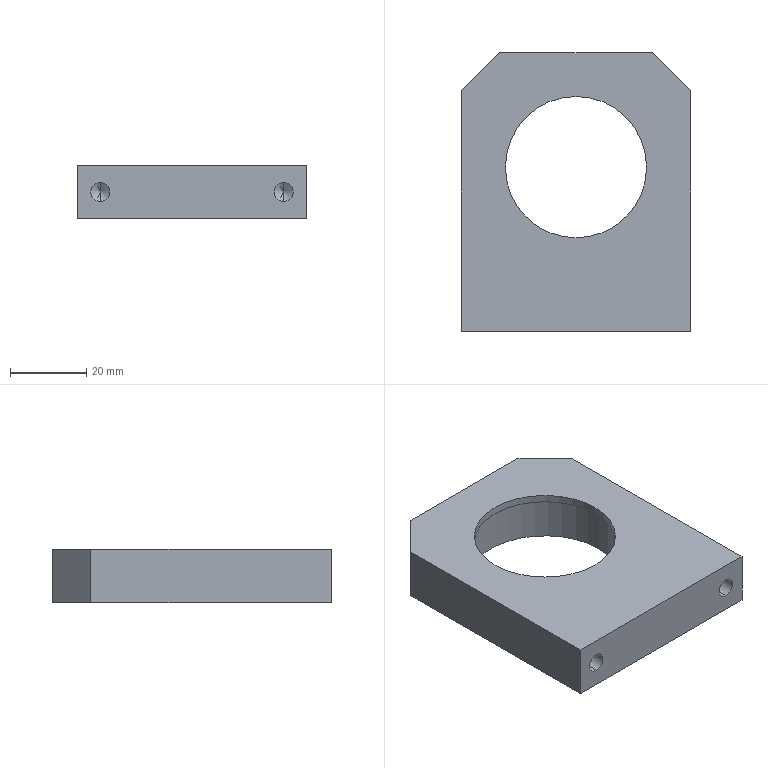Part | SolidWorks | features 3DProfileFeature 1, Chamfer 1, Extrusion 1, HoleWzd 1, ICE 1 | 1 solid | 21 faces | box 60 x 73 x 14 mm | volume 42120 mm3 | plane 9 | cylinder 8 | cone 4 | commonest cylinder face diameters 5 x4 37 x2 40 x2
STEP:
#1=CARTESIAN_POINT('',(-24.,-22.5,2.5));
#2=VERTEX_POINT('',#1);
#3=CARTESIAN_POINT('',(-24.,-22.5,-2.5));
#4=VERTEX_POINT('',#3);
#5=CARTESIAN_POINT('',(-24.,-22.5,0.));
#6=DIRECTION('',(0.,-1.,0.));
#7=DIRECTION('',(0.,0.,-1.));
#8=AXIS2_PLACEMENT_3D('',#5,#6,#7);
#9=CIRCLE('',#8,2.5);
#10=EDGE_CURVE('',#2,#4,#9,.T.);
#11=ORIENTED_EDGE('',*,*,#10,.F.);
#12=CARTESIAN_POINT('',(-24.,-36.5,2.5));
#13=VERTEX_POINT('',#12);
#14=CARTESIAN_POINT('',(-24.,-36.5,2.5));
#15=DIRECTION('',(0.,-1.,0.));
#16=VECTOR('',#15,1000.);
#17=LINE('',#14,#16);
#18=EDGE_CURVE('',#2,#13,#17,.T.);
#19=ORIENTED_EDGE('',*,*,#18,.T.);
#20=CARTESIAN_POINT('',(-24.,-36.5,-2.5));
#21=VERTEX_POINT('',#20);
#22=CARTESIAN_POINT('',(-24.,-36.5,0.));
#23=DIRECTION('',(0.,-1.,0.));
#24=DIRECTION('',(0.,0.,-1.));
#25=AXIS2_PLACEMENT_3D('',#22,#23,#24);
#26=CIRCLE('',#25,2.5);
#27=EDGE_CURVE('',#13,#21,#26,.T.);
#28=ORIENTED_EDGE('',*,*,#27,.T.);
#29=CARTESIAN_POINT('',(-24.,-36.5,-2.5));
#30=DIRECTION('',(0.,-1.,0.));
#31=VECTOR('',#30,1000.);
#32=LINE('',#29,#31);
#33=EDGE_CURVE('',#4,#21,#32,.T.);
#34=ORIENTED_EDGE('',*,*,#33,.F.);
#35=EDGE_LOOP('',(#11,#19,#28,#34));
#36=FACE_OUTER_BOUND('',#35,.T.);
#37=CARTESIAN_POINT('',(-24.,-36.5,0.));
#38=DIRECTION('',(0.,-1.,0.));
#39=DIRECTION('',(0.,0.,-1.));
#40=AXIS2_PLACEMENT_3D('',#37,#38,#39);
#41=CYLINDRICAL_SURFACE('',#40,2.5);
#42=ADVANCED_FACE('',(#36),#41,.F.);
#43=CARTESIAN_POINT('',(-24.,-20.998,0.));
#44=VERTEX_POINT('',#43);
#45=CARTESIAN_POINT('',(-24.,-22.5,-2.5));
#46=DIRECTION('',(0.,-0.515,-0.8572));
#47=VECTOR('',#46,1000.);
#48=LINE('',#45,#47);
#49=EDGE_CURVE('',#44,#4,#48,.T.);
#50=ORIENTED_EDGE('',*,*,#49,.F.);
#51=CARTESIAN_POINT('',(-24.,-22.5,2.5));
#52=DIRECTION('',(0.,-0.515,0.8572));
#53=VECTOR('',#52,1000.);
#54=LINE('',#51,#53);
#55=EDGE_CURVE('',#44,#2,#54,.T.);
#56=ORIENTED_EDGE('',*,*,#55,.T.);
#57=ORIENTED_EDGE('',*,*,#10,.T.);
#58=EDGE_LOOP('',(#50,#56,#57));
#59=FACE_OUTER_BOUND('',#58,.T.);
#60=CARTESIAN_POINT('',(-24.,-22.5,0.));
#61=DIRECTION('',(0.,-1.,0.));
#62=DIRECTION('',(0.,0.,-1.));
#63=AXIS2_PLACEMENT_3D('',#60,#61,#62);
#64=CONICAL_SURFACE('',#63,2.5,1.03);
#65=ADVANCED_FACE('',(#59),#64,.F.);
#66=CARTESIAN_POINT('',(24.,-22.5,2.5));
#67=VERTEX_POINT('',#66);
#68=CARTESIAN_POINT('',(24.,-22.5,-2.5));
#69=VERTEX_POINT('',#68);
#70=CARTESIAN_POINT('',(24.,-22.5,0.));
#71=DIRECTION('',(0.,-1.,0.));
#72=DIRECTION('',(0.,0.,-1.));
#73=AXIS2_PLACEMENT_3D('',#70,#71,#72);
#74=CIRCLE('',#73,2.5);
#75=EDGE_CURVE('',#67,#69,#74,.T.);
#76=ORIENTED_EDGE('',*,*,#75,.F.);
#77=CARTESIAN_POINT('',(24.,-36.5,2.5));
#78=VERTEX_POINT('',#77);
#79=CARTESIAN_POINT('',(24.,-36.5,2.5));
#80=DIRECTION('',(0.,-1.,0.));
#81=VECTOR('',#80,1000.);
#82=LINE('',#79,#81);
#83=EDGE_CURVE('',#67,#78,#82,.T.);
#84=ORIENTED_EDGE('',*,*,#83,.T.);
#85=CARTESIAN_POINT('',(24.,-36.5,-2.5));
#86=VERTEX_POINT('',#85);
#87=CARTESIAN_POINT('',(24.,-36.5,0.));
#88=DIRECTION('',(0.,-1.,0.));
#89=DIRECTION('',(0.,0.,-1.));
#90=AXIS2_PLACEMENT_3D('',#87,#88,#89);
#91=CIRCLE('',#90,2.5);
#92=EDGE_CURVE('',#78,#86,#91,.T.);
#93=ORIENTED_EDGE('',*,*,#92,.T.);
#94=CARTESIAN_POINT('',(24.,-36.5,-2.5));
#95=DIRECTION('',(0.,-1.,0.));
#96=VECTOR('',#95,1000.);
#97=LINE('',#94,#96);
#98=EDGE_CURVE('',#69,#86,#97,.T.);
#99=ORIENTED_EDGE('',*,*,#98,.F.);
#100=EDGE_LOOP('',(#76,#84,#93,#99));
#101=FACE_OUTER_BOUND('',#100,.T.);
#102=CARTESIAN_POINT('',(24.,-36.5,0.));
#103=DIRECTION('',(0.,-1.,0.));
#104=DIRECTION('',(0.,0.,-1.));
#105=AXIS2_PLACEMENT_3D('',#102,#103,#104);
#106=CYLINDRICAL_SURFACE('',#105,2.5);
#107=ADVANCED_FACE('',(#101),#106,.F.);
#108=CARTESIAN_POINT('',(24.,-20.998,0.));
#109=VERTEX_POINT('',#108);
#110=CARTESIAN_POINT('',(24.,-22.5,-2.5));
#111=DIRECTION('',(0.,-0.515,-0.8572));
#112=VECTOR('',#111,1000.);
#113=LINE('',#110,#112);
#114=EDGE_CURVE('',#109,#69,#113,.T.);
#115=ORIENTED_EDGE('',*,*,#114,.F.);
#116=CARTESIAN_POINT('',(24.,-22.5,2.5));
#117=DIRECTION('',(0.,-0.515,0.8572));
#118=VECTOR('',#117,1000.);
#119=LINE('',#116,#118);
#120=EDGE_CURVE('',#109,#67,#119,.T.);
#121=ORIENTED_EDGE('',*,*,#120,.T.);
#122=ORIENTED_EDGE('',*,*,#75,.T.);
#123=EDGE_LOOP('',(#115,#121,#122));
#124=FACE_OUTER_BOUND('',#123,.T.);
#125=CARTESIAN_POINT('',(24.,-22.5,0.));
#126=DIRECTION('',(0.,-1.,0.));
#127=DIRECTION('',(0.,0.,-1.));
#128=AXIS2_PLACEMENT_3D('',#125,#126,#127);
#129=CONICAL_SURFACE('',#128,2.5,1.03);
#130=ADVANCED_FACE('',(#124),#129,.F.);
#131=CARTESIAN_POINT('',(-18.5,6.5,5.));
#132=VERTEX_POINT('',#131);
#133=CARTESIAN_POINT('',(18.5,6.5,5.));
#134=VERTEX_POINT('',#133);
#135=CARTESIAN_POINT('',(0.,6.5,5.));
#136=DIRECTION('',(0.,0.,1.));
#137=DIRECTION('',(1.,0.,0.));
#138=AXIS2_PLACEMENT_3D('',#135,#136,#137);
#139=CIRCLE('',#138,18.5);
#140=EDGE_CURVE('',#132,#134,#139,.T.);
#141=ORIENTED_EDGE('',*,*,#140,.F.);
#142=CARTESIAN_POINT('',(-18.5,6.5,7.));
#143=VERTEX_POINT('',#142);
#144=CARTESIAN_POINT('',(-18.5,6.5,5.));
#145=DIRECTION('',(0.,0.,1.));
#146=VECTOR('',#145,1000.);
#147=LINE('',#144,#146);
#148=EDGE_CURVE('',#132,#143,#147,.T.);
#149=ORIENTED_EDGE('',*,*,#148,.T.);
#150=CARTESIAN_POINT('',(18.5,6.5,7.));
#151=VERTEX_POINT('',#150);
#152=CARTESIAN_POINT('',(0.,6.5,7.));
#153=DIRECTION('',(0.,0.,1.));
#154=DIRECTION('',(1.,0.,0.));
#155=AXIS2_PLACEMENT_3D('',#152,#153,#154);
#156=CIRCLE('',#155,18.5);
#157=EDGE_CURVE('',#143,#151,#156,.T.);
#158=ORIENTED_EDGE('',*,*,#157,.T.);
#159=CARTESIAN_POINT('',(18.5,6.5,5.));
#160=DIRECTION('',(0.,0.,1.));
#161=VECTOR('',#160,1000.);
#162=LINE('',#159,#161);
#163=EDGE_CURVE('',#134,#151,#162,.T.);
#164=ORIENTED_EDGE('',*,*,#163,.F.);
#165=EDGE_LOOP('',(#141,#149,#158,#164));
#166=FACE_OUTER_BOUND('',#165,.T.);
#167=CARTESIAN_POINT('',(0.,6.5,5.));
#168=DIRECTION('',(0.,0.,1.));
#169=DIRECTION('',(1.,0.,0.));
#170=AXIS2_PLACEMENT_3D('',#167,#168,#169);
#171=CYLINDRICAL_SURFACE('',#170,18.5);
#172=ADVANCED_FACE('',(#166),#171,.F.);
#173=CARTESIAN_POINT('',(-20.,6.5,5.));
#174=VERTEX_POINT('',#173);
#175=CARTESIAN_POINT('',(20.,6.5,5.));
#176=VERTEX_POINT('',#175);
#177=CARTESIAN_POINT('',(0.,6.5,5.));
#178=DIRECTION('',(0.,0.,1.));
#179=DIRECTION('',(1.,0.,0.));
#180=AXIS2_PLACEMENT_3D('',#177,#178,#179);
#181=CIRCLE('',#180,20.);
#182=EDGE_CURVE('',#174,#176,#181,.T.);
#183=ORIENTED_EDGE('',*,*,#182,.T.);
#184=CARTESIAN_POINT('',(20.,6.5,-7.));
#185=VERTEX_POINT('',#184);
#186=CARTESIAN_POINT('',(20.,6.5,7.));
#187=DIRECTION('',(0.,0.,-1.));
#188=VECTOR('',#187,1000.);
#189=LINE('',#186,#188);
#190=EDGE_CURVE('',#176,#185,#189,.T.);
#191=ORIENTED_EDGE('',*,*,#190,.T.);
#192=CARTESIAN_POINT('',(-20.,6.5,-7.));
#193=VERTEX_POINT('',#192);
#194=CARTESIAN_POINT('',(0.,6.5,-7.));
#195=DIRECTION('',(0.,0.,1.));
#196=DIRECTION('',(1.,0.,0.));
#197=AXIS2_PLACEMENT_3D('',#194,#195,#196);
#198=CIRCLE('',#197,20.);
#199=EDGE_CURVE('',#193,#185,#198,.T.);
#200=ORIENTED_EDGE('',*,*,#199,.F.);
#201=CARTESIAN_POINT('',(-20.,6.5,7.));
#202=DIRECTION('',(0.,0.,-1.));
#203=VECTOR('',#202,1000.);
#204=LINE('',#201,#203);
#205=EDGE_CURVE('',#174,#193,#204,.T.);
#206=ORIENTED_EDGE('',*,*,#205,.F.);
#207=EDGE_LOOP('',(#183,#191,#200,#206));
#208=FACE_OUTER_BOUND('',#207,.T.);
#209=CARTESIAN_POINT('',(0.,6.5,7.));
#210=DIRECTION('',(0.,0.,-1.));
#211=DIRECTION('',(-1.,0.,0.));
#212=AXIS2_PLACEMENT_3D('',#209,#210,#211);
#213=CYLINDRICAL_SURFACE('',#212,20.);
#214=ADVANCED_FACE('',(#208),#213,.F.);
#215=ORIENTED_EDGE('',*,*,#190,.F.);
#216=CARTESIAN_POINT('',(0.,6.5,5.));
#217=DIRECTION('',(0.,0.,1.));
#218=DIRECTION('',(1.,0.,0.));
#219=AXIS2_PLACEMENT_3D('',#216,#217,#218);
#220=CIRCLE('',#219,20.);
#221=EDGE_CURVE('',#176,#174,#220,.T.);
#222=ORIENTED_EDGE('',*,*,#221,.T.);
#223=ORIENTED_EDGE('',*,*,#205,.T.);
#224=CARTESIAN_POINT('',(0.,6.5,-7.));
#225=DIRECTION('',(0.,0.,1.));
#226=DIRECTION('',(1.,0.,0.));
#227=AXIS2_PLACEMENT_3D('',#224,#225,#226);
#228=CIRCLE('',#227,20.);
#229=EDGE_CURVE('',#185,#193,#228,.T.);
#230=ORIENTED_EDGE('',*,*,#229,.F.);
#231=EDGE_LOOP('',(#215,#222,#223,#230));
#232=FACE_OUTER_BOUND('',#231,.T.);
#233=CARTESIAN_POINT('',(0.,6.5,7.));
#234=DIRECTION('',(0.,0.,-1.));
#235=DIRECTION('',(-1.,0.,0.));
#236=AXIS2_PLACEMENT_3D('',#233,#234,#235);
#237=CYLINDRICAL_SURFACE('',#236,20.);
#238=ADVANCED_FACE('',(#232),#237,.F.);
#239=CARTESIAN_POINT('',(30.,-36.5,7.));
#240=VERTEX_POINT('',#239);
#241=CARTESIAN_POINT('',(30.,26.5,7.));
#242=VERTEX_POINT('',#241);
#243=CARTESIAN_POINT('',(30.,-36.5,7.));
#244=DIRECTION('',(0.,1.,0.));
#245=VECTOR('',#244,1000.);
#246=LINE('',#243,#245);
#247=EDGE_CURVE('',#240,#242,#246,.T.);
#248=ORIENTED_EDGE('',*,*,#247,.T.);
#249=CARTESIAN_POINT('',(20.,36.5,7.));
#250=VERTEX_POINT('',#249);
#251=CARTESIAN_POINT('',(20.,36.5,7.));
#252=DIRECTION('',(-0.7071,0.7071,0.));
#253=VECTOR('',#252,1000.);
#254=LINE('',#251,#253);
#255=EDGE_CURVE('',#242,#250,#254,.T.);
#256=ORIENTED_EDGE('',*,*,#255,.T.);
#257=CARTESIAN_POINT('',(-20.,36.5,7.));
#258=VERTEX_POINT('',#257);
#259=CARTESIAN_POINT('',(-30.,36.5,7.));
#260=DIRECTION('',(-1.,0.,0.));
#261=VECTOR('',#260,1000.);
#262=LINE('',#259,#261);
#263=EDGE_CURVE('',#250,#258,#262,.T.);
#264=ORIENTED_EDGE('',*,*,#263,.T.);
#265=CARTESIAN_POINT('',(-30.,26.5,7.));
#266=VERTEX_POINT('',#265);
#267=CARTESIAN_POINT('',(-30.,26.5,7.));
#268=DIRECTION('',(-0.7071,-0.7071,0.));
#269=VECTOR('',#268,1000.);
#270=LINE('',#267,#269);
#271=EDGE_CURVE('',#258,#266,#270,.T.);
#272=ORIENTED_EDGE('',*,*,#271,.T.);
#273=CARTESIAN_POINT('',(-30.,-36.5,7.));
#274=VERTEX_POINT('',#273);
#275=CARTESIAN_POINT('',(-30.,-36.5,7.));
#276=DIRECTION('',(0.,-1.,0.));
#277=VECTOR('',#276,1000.);
#278=LINE('',#275,#277);
#279=EDGE_CURVE('',#266,#274,#278,.T.);
#280=ORIENTED_EDGE('',*,*,#279,.T.);
#281=CARTESIAN_POINT('',(-30.,-36.5,7.));
#282=DIRECTION('',(1.,0.,0.));
#283=VECTOR('',#282,1000.);
#284=LINE('',#281,#283);
#285=EDGE_CURVE('',#274,#240,#284,.T.);
#286=ORIENTED_EDGE('',*,*,#285,.T.);
#287=EDGE_LOOP('',(#248,#256,#264,#272,#280,#286));
#288=FACE_OUTER_BOUND('',#287,.T.);
#289=CARTESIAN_POINT('',(0.,6.5,7.));
#290=DIRECTION('',(0.,0.,1.));
#291=DIRECTION('',(1.,0.,0.));
#292=AXIS2_PLACEMENT_3D('',#289,#290,#291);
#293=CIRCLE('',#292,18.5);
#294=EDGE_CURVE('',#151,#143,#293,.T.);
#295=ORIENTED_EDGE('',*,*,#294,.F.);
#296=ORIENTED_EDGE('',*,*,#157,.F.);
#297=EDGE_LOOP('',(#295,#296));
#298=FACE_BOUND('',#297,.T.);
#299=CARTESIAN_POINT('',(0.,0.,7.));
#300=DIRECTION('',(0.,0.,-1.));
#301=DIRECTION('',(-1.,0.,0.));
#302=AXIS2_PLACEMENT_3D('',#299,#300,#301);
#303=PLANE('',#302);
#304=ADVANCED_FACE('',(#288,#298),#303,.F.);
#305=CARTESIAN_POINT('',(20.,36.5,-7.));
#306=VERTEX_POINT('',#305);
#307=CARTESIAN_POINT('',(-20.,36.5,-7.));
#308=VERTEX_POINT('',#307);
#309=CARTESIAN_POINT('',(-30.,36.5,-7.));
#310=DIRECTION('',(-1.,0.,0.));
#311=VECTOR('',#310,1000.);
#312=LINE('',#309,#311);
#313=EDGE_CURVE('',#306,#308,#312,.T.);
#314=ORIENTED_EDGE('',*,*,#313,.F.);
#315=CARTESIAN_POINT('',(30.,26.5,-7.));
#316=VERTEX_POINT('',#315);
#317=CARTESIAN_POINT('',(28.25,28.25,-7.));
#318=DIRECTION('',(0.7071,-0.7071,0.));
#319=VECTOR('',#318,1000.);
#320=LINE('',#317,#319);
#321=EDGE_CURVE('',#306,#316,#320,.T.);
#322=ORIENTED_EDGE('',*,*,#321,.T.);
#323=CARTESIAN_POINT('',(30.,-36.5,-7.));
#324=VERTEX_POINT('',#323);
#325=CARTESIAN_POINT('',(30.,-36.5,-7.));
#326=DIRECTION('',(0.,1.,0.));
#327=VECTOR('',#326,1000.);
#328=LINE('',#325,#327);
#329=EDGE_CURVE('',#324,#316,#328,.T.);
#330=ORIENTED_EDGE('',*,*,#329,.F.);
#331=CARTESIAN_POINT('',(-30.,-36.5,-7.));
#332=VERTEX_POINT('',#331);
#333=CARTESIAN_POINT('',(-30.,-36.5,-7.));
#334=DIRECTION('',(1.,0.,0.));
#335=VECTOR('',#334,1000.);
#336=LINE('',#333,#335);
#337=EDGE_CURVE('',#332,#324,#336,.T.);
#338=ORIENTED_EDGE('',*,*,#337,.F.);
#339=CARTESIAN_POINT('',(-30.,26.5,-7.));
#340=VERTEX_POINT('',#339);
#341=CARTESIAN_POINT('',(-30.,-36.5,-7.));
#342=DIRECTION('',(0.,-1.,0.));
#343=VECTOR('',#342,1000.);
#344=LINE('',#341,#343);
#345=EDGE_CURVE('',#340,#332,#344,.T.);
#346=ORIENTED_EDGE('',*,*,#345,.F.);
#347=CARTESIAN_POINT('',(-28.25,28.25,-7.));
#348=DIRECTION('',(0.7071,0.7071,0.));
#349=VECTOR('',#348,1000.);
#350=LINE('',#347,#349);
#351=EDGE_CURVE('',#340,#308,#350,.T.);
#352=ORIENTED_EDGE('',*,*,#351,.T.);
#353=EDGE_LOOP('',(#314,#322,#330,#338,#346,#352));
#354=FACE_OUTER_BOUND('',#353,.T.);
#355=ORIENTED_EDGE('',*,*,#199,.T.);
#356=ORIENTED_EDGE('',*,*,#229,.T.);
#357=EDGE_LOOP('',(#355,#356));
#358=FACE_BOUND('',#357,.T.);
#359=CARTESIAN_POINT('',(0.,0.,-7.));
#360=DIRECTION('',(0.,0.,-1.));
#361=DIRECTION('',(-1.,0.,0.));
#362=AXIS2_PLACEMENT_3D('',#359,#360,#361);
#363=PLANE('',#362);
#364=ADVANCED_FACE('',(#354,#358),#363,.T.);
#365=ORIENTED_EDGE('',*,*,#329,.T.);
#366=CARTESIAN_POINT('',(30.,26.5,7.));
#367=DIRECTION('',(0.,0.,1.));
#368=VECTOR('',#367,1000.);
#369=LINE('',#366,#368);
#370=EDGE_CURVE('',#316,#242,#369,.T.);
#371=ORIENTED_EDGE('',*,*,#370,.T.);
#372=ORIENTED_EDGE('',*,*,#247,.F.);
#373=CARTESIAN_POINT('',(30.,-36.5,7.));
#374=DIRECTION('',(0.,0.,-1.));
#375=VECTOR('',#374,1000.);
#376=LINE('',#373,#375);
#377=EDGE_CURVE('',#240,#324,#376,.T.);
#378=ORIENTED_EDGE('',*,*,#377,.T.);
#379=EDGE_LOOP('',(#365,#371,#372,#378));
#380=FACE_OUTER_BOUND('',#379,.T.);
#381=CARTESIAN_POINT('',(30.,-36.5,7.));
#382=DIRECTION('',(-1.,0.,0.));
#383=DIRECTION('',(0.,0.,1.));
#384=AXIS2_PLACEMENT_3D('',#381,#382,#383);
#385=PLANE('',#384);
#386=ADVANCED_FACE('',(#380),#385,.F.);
#387=ORIENTED_EDGE('',*,*,#263,.F.);
#388=CARTESIAN_POINT('',(20.,36.5,7.));
#389=DIRECTION('',(0.,0.,-1.));
#390=VECTOR('',#389,1000.);
#391=LINE('',#388,#390);
#392=EDGE_CURVE('',#250,#306,#391,.T.);
#393=ORIENTED_EDGE('',*,*,#392,.T.);
#394=ORIENTED_EDGE('',*,*,#313,.T.);
#395=CARTESIAN_POINT('',(-20.,36.5,7.));
#396=DIRECTION('',(0.,0.,1.));
#397=VECTOR('',#396,1000.);
#398=LINE('',#395,#397);
#399=EDGE_CURVE('',#308,#258,#398,.T.);
#400=ORIENTED_EDGE('',*,*,#399,.T.);
#401=EDGE_LOOP('',(#387,#393,#394,#400));
#402=FACE_OUTER_BOUND('',#401,.T.);
#403=CARTESIAN_POINT('',(-30.,36.5,7.));
#404=DIRECTION('',(0.,-1.,0.));
#405=DIRECTION('',(1.,0.,0.));
#406=AXIS2_PLACEMENT_3D('',#403,#404,#405);
#407=PLANE('',#406);
#408=ADVANCED_FACE('',(#402),#407,.F.);
#409=ORIENTED_EDGE('',*,*,#279,.F.);
#410=CARTESIAN_POINT('',(-30.,26.5,7.));
#411=DIRECTION('',(0.,0.,-1.));
#412=VECTOR('',#411,1000.);
#413=LINE('',#410,#412);
#414=EDGE_CURVE('',#266,#340,#413,.T.);
#415=ORIENTED_EDGE('',*,*,#414,.T.);
#416=ORIENTED_EDGE('',*,*,#345,.T.);
#417=CARTESIAN_POINT('',(-30.,-36.5,7.));
#418=DIRECTION('',(0.,0.,-1.));
#419=VECTOR('',#418,1000.);
#420=LINE('',#417,#419);
#421=EDGE_CURVE('',#274,#332,#420,.T.);
#422=ORIENTED_EDGE('',*,*,#421,.F.);
#423=EDGE_LOOP('',(#409,#415,#416,#422));
#424=FACE_OUTER_BOUND('',#423,.T.);
#425=CARTESIAN_POINT('',(-30.,-36.5,7.));
#426=DIRECTION('',(1.,0.,0.));
#427=DIRECTION('',(0.,0.,-1.));
#428=AXIS2_PLACEMENT_3D('',#425,#426,#427);
#429=PLANE('',#428);
#430=ADVANCED_FACE('',(#424),#429,.F.);
#431=CARTESIAN_POINT('',(-24.,-36.5,0.));
#432=DIRECTION('',(0.,-1.,0.));
#433=DIRECTION('',(0.,0.,-1.));
#434=AXIS2_PLACEMENT_3D('',#431,#432,#433);
#435=CIRCLE('',#434,2.5);
#436=EDGE_CURVE('',#21,#13,#435,.T.);
#437=ORIENTED_EDGE('',*,*,#436,.F.);
#438=ORIENTED_EDGE('',*,*,#27,.F.);
#439=EDGE_LOOP('',(#437,#438));
#440=FACE_BOUND('',#439,.T.);
#441=CARTESIAN_POINT('',(24.,-36.5,0.));
#442=DIRECTION('',(0.,-1.,0.));
#443=DIRECTION('',(0.,0.,-1.));
#444=AXIS2_PLACEMENT_3D('',#441,#442,#443);
#445=CIRCLE('',#444,2.5);
#446=EDGE_CURVE('',#86,#78,#445,.T.);
#447=ORIENTED_EDGE('',*,*,#446,.F.);
#448=ORIENTED_EDGE('',*,*,#92,.F.);
#449=EDGE_LOOP('',(#447,#448));
#450=FACE_BOUND('',#449,.T.);
#451=ORIENTED_EDGE('',*,*,#337,.T.);
#452=ORIENTED_EDGE('',*,*,#377,.F.);
#453=ORIENTED_EDGE('',*,*,#285,.F.);
#454=ORIENTED_EDGE('',*,*,#421,.T.);
#455=EDGE_LOOP('',(#451,#452,#453,#454));
#456=FACE_OUTER_BOUND('',#455,.T.);
#457=CARTESIAN_POINT('',(-30.,-36.5,7.));
#458=DIRECTION('',(0.,1.,0.));
#459=DIRECTION('',(0.,0.,1.));
#460=AXIS2_PLACEMENT_3D('',#457,#458,#459);
#461=PLANE('',#460);
#462=ADVANCED_FACE('',(#440,#450,#456),#461,.F.);
#463=CARTESIAN_POINT('',(0.,6.5,5.));
#464=DIRECTION('',(0.,0.,1.));
#465=DIRECTION('',(1.,0.,0.));
#466=AXIS2_PLACEMENT_3D('',#463,#464,#465);
#467=CIRCLE('',#466,18.5);
#468=EDGE_CURVE('',#134,#132,#467,.T.);
#469=ORIENTED_EDGE('',*,*,#468,.T.);
#470=ORIENTED_EDGE('',*,*,#140,.T.);
#471=EDGE_LOOP('',(#469,#470));
#472=FACE_BOUND('',#471,.T.);
#473=ORIENTED_EDGE('',*,*,#182,.F.);
#474=ORIENTED_EDGE('',*,*,#221,.F.);
#475=EDGE_LOOP('',(#473,#474));
#476=FACE_OUTER_BOUND('',#475,.T.);
#477=CARTESIAN_POINT('',(0.,6.5,5.));
#478=DIRECTION('',(0.,0.,1.));
#479=DIRECTION('',(1.,0.,0.));
#480=AXIS2_PLACEMENT_3D('',#477,#478,#479);
#481=PLANE('',#480);
#482=ADVANCED_FACE('',(#472,#476),#481,.F.);
#483=ORIENTED_EDGE('',*,*,#148,.F.);
#484=ORIENTED_EDGE('',*,*,#468,.F.);
#485=ORIENTED_EDGE('',*,*,#163,.T.);
#486=ORIENTED_EDGE('',*,*,#294,.T.);
#487=EDGE_LOOP('',(#483,#484,#485,#486));
#488=FACE_OUTER_BOUND('',#487,.T.);
#489=CARTESIAN_POINT('',(0.,6.5,5.));
#490=DIRECTION('',(0.,0.,1.));
#491=DIRECTION('',(1.,0.,0.));
#492=AXIS2_PLACEMENT_3D('',#489,#490,#491);
#493=CYLINDRICAL_SURFACE('',#492,18.5);
#494=ADVANCED_FACE('',(#488),#493,.F.);
#495=ORIENTED_EDGE('',*,*,#255,.F.);
#496=ORIENTED_EDGE('',*,*,#370,.F.);
#497=ORIENTED_EDGE('',*,*,#321,.F.);
#498=ORIENTED_EDGE('',*,*,#392,.F.);
#499=EDGE_LOOP('',(#495,#496,#497,#498));
#500=FACE_OUTER_BOUND('',#499,.T.);
#501=CARTESIAN_POINT('',(20.,36.5,7.));
#502=DIRECTION('',(-0.7071,-0.7071,0.));
#503=DIRECTION('',(0.,0.,-1.));
#504=AXIS2_PLACEMENT_3D('',#501,#502,#503);
#505=PLANE('',#504);
#506=ADVANCED_FACE('',(#500),#505,.F.);
#507=ORIENTED_EDGE('',*,*,#271,.F.);
#508=ORIENTED_EDGE('',*,*,#399,.F.);
#509=ORIENTED_EDGE('',*,*,#351,.F.);
#510=ORIENTED_EDGE('',*,*,#414,.F.);
#511=EDGE_LOOP('',(#507,#508,#509,#510));
#512=FACE_OUTER_BOUND('',#511,.T.);
#513=CARTESIAN_POINT('',(-30.,26.5,7.));
#514=DIRECTION('',(0.7071,-0.7071,0.));
#515=DIRECTION('',(0.,0.,-1.));
#516=AXIS2_PLACEMENT_3D('',#513,#514,#515);
#517=PLANE('',#516);
#518=ADVANCED_FACE('',(#512),#517,.F.);
#519=ORIENTED_EDGE('',*,*,#120,.F.);
#520=ORIENTED_EDGE('',*,*,#114,.T.);
#521=CARTESIAN_POINT('',(24.,-22.5,0.));
#522=DIRECTION('',(0.,-1.,0.));
#523=DIRECTION('',(0.,0.,-1.));
#524=AXIS2_PLACEMENT_3D('',#521,#522,#523);
#525=CIRCLE('',#524,2.5);
#526=EDGE_CURVE('',#69,#67,#525,.T.);
#527=ORIENTED_EDGE('',*,*,#526,.T.);
#528=EDGE_LOOP('',(#519,#520,#527));
#529=FACE_OUTER_BOUND('',#528,.T.);
#530=CARTESIAN_POINT('',(24.,-22.5,0.));
#531=DIRECTION('',(0.,-1.,0.));
#532=DIRECTION('',(0.,0.,-1.));
#533=AXIS2_PLACEMENT_3D('',#530,#531,#532);
#534=CONICAL_SURFACE('',#533,2.5,1.03);
#535=ADVANCED_FACE('',(#529),#534,.F.);
#536=ORIENTED_EDGE('',*,*,#83,.F.);
#537=ORIENTED_EDGE('',*,*,#526,.F.);
#538=ORIENTED_EDGE('',*,*,#98,.T.);
#539=ORIENTED_EDGE('',*,*,#446,.T.);
#540=EDGE_LOOP('',(#536,#537,#538,#539));
#541=FACE_OUTER_BOUND('',#540,.T.);
#542=CARTESIAN_POINT('',(24.,-36.5,0.));
#543=DIRECTION('',(0.,-1.,0.));
#544=DIRECTION('',(0.,0.,-1.));
#545=AXIS2_PLACEMENT_3D('',#542,#543,#544);
#546=CYLINDRICAL_SURFACE('',#545,2.5);
#547=ADVANCED_FACE('',(#541),#546,.F.);
#548=ORIENTED_EDGE('',*,*,#55,.F.);
#549=ORIENTED_EDGE('',*,*,#49,.T.);
#550=CARTESIAN_POINT('',(-24.,-22.5,0.));
#551=DIRECTION('',(0.,-1.,0.));
#552=DIRECTION('',(0.,0.,-1.));
#553=AXIS2_PLACEMENT_3D('',#550,#551,#552);
#554=CIRCLE('',#553,2.5);
#555=EDGE_CURVE('',#4,#2,#554,.T.);
#556=ORIENTED_EDGE('',*,*,#555,.T.);
#557=EDGE_LOOP('',(#548,#549,#556));
#558=FACE_OUTER_BOUND('',#557,.T.);
#559=CARTESIAN_POINT('',(-24.,-22.5,0.));
#560=DIRECTION('',(0.,-1.,0.));
#561=DIRECTION('',(0.,0.,-1.));
#562=AXIS2_PLACEMENT_3D('',#559,#560,#561);
#563=CONICAL_SURFACE('',#562,2.5,1.03);
#564=ADVANCED_FACE('',(#558),#563,.F.);
#565=ORIENTED_EDGE('',*,*,#18,.F.);
#566=ORIENTED_EDGE('',*,*,#555,.F.);
#567=ORIENTED_EDGE('',*,*,#33,.T.);
#568=ORIENTED_EDGE('',*,*,#436,.T.);
#569=EDGE_LOOP('',(#565,#566,#567,#568));
#570=FACE_OUTER_BOUND('',#569,.T.);
#571=CARTESIAN_POINT('',(-24.,-36.5,0.));
#572=DIRECTION('',(0.,-1.,0.));
#573=DIRECTION('',(0.,0.,-1.));
#574=AXIS2_PLACEMENT_3D('',#571,#572,#573);
#575=CYLINDRICAL_SURFACE('',#574,2.5);
#576=ADVANCED_FACE('',(#570),#575,.F.);
#577=CLOSED_SHELL('',(#42,#65,#107,#130,#172,#214,#238,#304,#364,#386,#408,#430,#462,#482,#494,#506,#518,#535,#547,#564,#576));
#578=MANIFOLD_SOLID_BREP('',#577);
#579=CARTESIAN_POINT('',(0.,0.,0.));
#580=DIRECTION('',(0.,0.,1.));
#581=DIRECTION('',(1.,0.,0.));
#582=AXIS2_PLACEMENT_3D('',#579,#580,#581);
#583=(LENGTH_UNIT()NAMED_UNIT(*)SI_UNIT(.MILLI.,.METRE.));
#584=UNCERTAINTY_MEASURE_WITH_UNIT(LENGTH_MEASURE(0.00001),#583,'','');
#585=(NAMED_UNIT(*)PLANE_ANGLE_UNIT()SI_UNIT($,.RADIAN.));
#586=(NAMED_UNIT(*)SI_UNIT($,.STERADIAN.)SOLID_ANGLE_UNIT());
#587=(GEOMETRIC_REPRESENTATION_CONTEXT(3)GLOBAL_UNCERTAINTY_ASSIGNED_CONTEXT((#584))GLOBAL_UNIT_ASSIGNED_CONTEXT((#583,#585,#586))REPRESENTATION_CONTEXT('',''));
#588=ADVANCED_BREP_SHAPE_REPRESENTATION('',(#578,#582),#587);